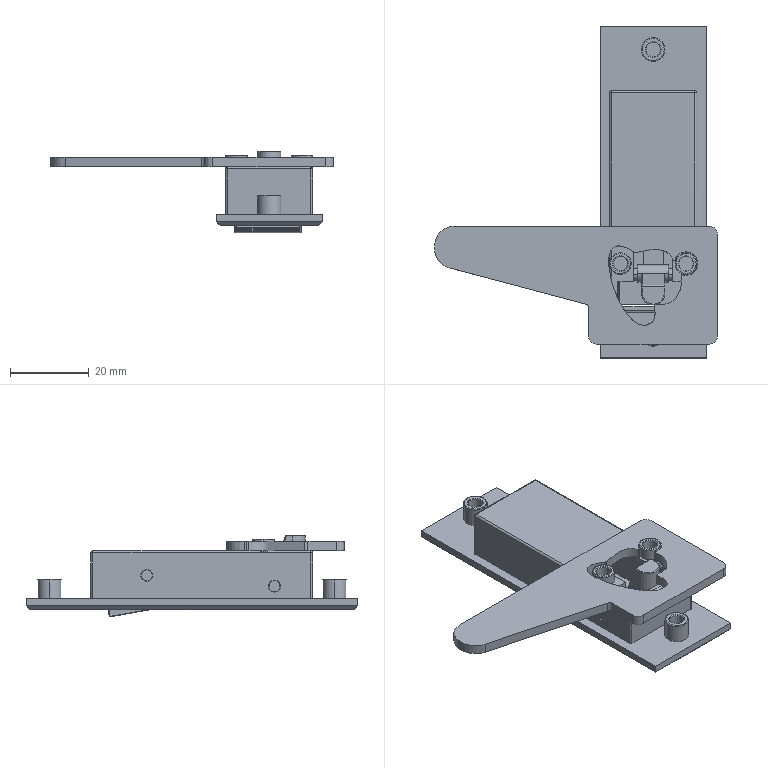Part | SolidWorks | 6 solids | 405 faces | box 72 x 84.5 x 20.798 mm | volume 17145 mm3 | plane 238 | cylinder 105 | spline 44 | cone 16 | torus 2 | commonest cylinder face diameters 0.4 x31 3 x16 0.2 x11 1 x11 3.6 x8 4 x8